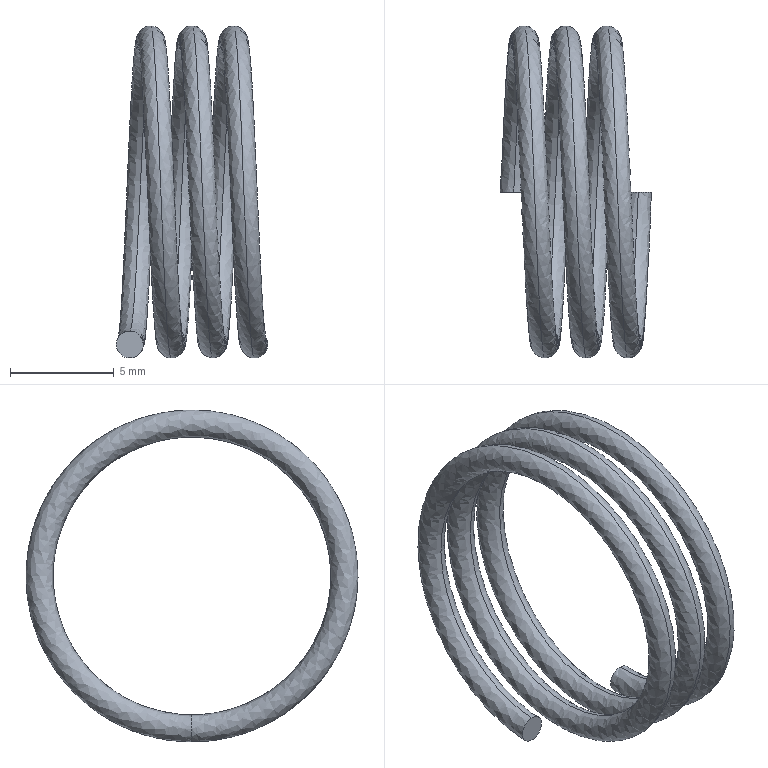Part | SolidWorks | features BaseBody 1, RefAxis 1 | 1 solid | 4 faces | box 7.3 x 16 x 16 mm | volume 183.83 mm3 | spline 2 | plane 2
STEP:
#1=CARTESIAN_POINT('',(-6.,0.,-8.));
#2=VERTEX_POINT('',#1);
#3=CARTESIAN_POINT('',(0.,0.,-8.));
#4=VERTEX_POINT('',#3);
#5=CARTESIAN_POINT('',(-6.,0.,-8.));
#6=CARTESIAN_POINT('',(-5.934,1.704,-8.));
#7=CARTESIAN_POINT('',(-5.866,3.324,-7.474));
#8=CARTESIAN_POINT('',(-5.8,4.702,-6.472));
#9=CARTESIAN_POINT('',(-5.734,6.081,-5.471));
#10=CARTESIAN_POINT('',(-5.666,7.082,-4.092));
#11=CARTESIAN_POINT('',(-5.6,7.608,-2.472));
#12=CARTESIAN_POINT('',(-5.534,8.135,-0.8518));
#13=CARTESIAN_POINT('',(-5.466,8.135,0.8518));
#14=CARTESIAN_POINT('',(-5.4,7.608,2.472));
#15=CARTESIAN_POINT('',(-5.334,7.082,4.092));
#16=CARTESIAN_POINT('',(-5.266,6.081,5.471));
#17=CARTESIAN_POINT('',(-5.2,4.702,6.472));
#18=CARTESIAN_POINT('',(-5.134,3.324,7.474));
#19=CARTESIAN_POINT('',(-5.066,1.704,8.));
#20=CARTESIAN_POINT('',(-5.,0.,8.));
#21=CARTESIAN_POINT('',(-4.934,-1.704,8.));
#22=CARTESIAN_POINT('',(-4.866,-3.324,7.474));
#23=CARTESIAN_POINT('',(-4.8,-4.702,6.472));
#24=CARTESIAN_POINT('',(-4.734,-6.081,5.471));
#25=CARTESIAN_POINT('',(-4.666,-7.082,4.092));
#26=CARTESIAN_POINT('',(-4.6,-7.608,2.472));
#27=CARTESIAN_POINT('',(-4.534,-8.135,0.8518));
#28=CARTESIAN_POINT('',(-4.466,-8.135,-0.8518));
#29=CARTESIAN_POINT('',(-4.4,-7.608,-2.472));
#30=CARTESIAN_POINT('',(-4.334,-7.082,-4.092));
#31=CARTESIAN_POINT('',(-4.266,-6.081,-5.471));
#32=CARTESIAN_POINT('',(-4.2,-4.702,-6.472));
#33=CARTESIAN_POINT('',(-4.134,-3.324,-7.474));
#34=CARTESIAN_POINT('',(-4.066,-1.704,-8.));
#35=CARTESIAN_POINT('',(-4.,0.,-8.));
#36=CARTESIAN_POINT('',(-3.934,1.704,-8.));
#37=CARTESIAN_POINT('',(-3.866,3.324,-7.474));
#38=CARTESIAN_POINT('',(-3.8,4.702,-6.472));
#39=CARTESIAN_POINT('',(-3.734,6.081,-5.471));
#40=CARTESIAN_POINT('',(-3.666,7.082,-4.092));
#41=CARTESIAN_POINT('',(-3.6,7.608,-2.472));
#42=CARTESIAN_POINT('',(-3.534,8.135,-0.8518));
#43=CARTESIAN_POINT('',(-3.466,8.135,0.8518));
#44=CARTESIAN_POINT('',(-3.4,7.608,2.472));
#45=CARTESIAN_POINT('',(-3.334,7.082,4.092));
#46=CARTESIAN_POINT('',(-3.266,6.081,5.471));
#47=CARTESIAN_POINT('',(-3.2,4.702,6.472));
#48=CARTESIAN_POINT('',(-3.134,3.324,7.474));
#49=CARTESIAN_POINT('',(-3.066,1.704,8.));
#50=CARTESIAN_POINT('',(-3.,0.,8.));
#51=CARTESIAN_POINT('',(-2.934,-1.704,8.));
#52=CARTESIAN_POINT('',(-2.866,-3.324,7.474));
#53=CARTESIAN_POINT('',(-2.8,-4.702,6.472));
#54=CARTESIAN_POINT('',(-2.734,-6.081,5.471));
#55=CARTESIAN_POINT('',(-2.666,-7.082,4.092));
#56=CARTESIAN_POINT('',(-2.6,-7.608,2.472));
#57=CARTESIAN_POINT('',(-2.534,-8.135,0.8518));
#58=CARTESIAN_POINT('',(-2.466,-8.135,-0.8518));
#59=CARTESIAN_POINT('',(-2.4,-7.608,-2.472));
#60=CARTESIAN_POINT('',(-2.334,-7.082,-4.092));
#61=CARTESIAN_POINT('',(-2.266,-6.081,-5.471));
#62=CARTESIAN_POINT('',(-2.2,-4.702,-6.472));
#63=CARTESIAN_POINT('',(-2.134,-3.324,-7.474));
#64=CARTESIAN_POINT('',(-2.066,-1.704,-8.));
#65=CARTESIAN_POINT('',(-2.,0.,-8.));
#66=CARTESIAN_POINT('',(-1.934,1.704,-8.));
#67=CARTESIAN_POINT('',(-1.866,3.324,-7.474));
#68=CARTESIAN_POINT('',(-1.8,4.702,-6.472));
#69=CARTESIAN_POINT('',(-1.734,6.081,-5.471));
#70=CARTESIAN_POINT('',(-1.666,7.082,-4.092));
#71=CARTESIAN_POINT('',(-1.6,7.608,-2.472));
#72=CARTESIAN_POINT('',(-1.534,8.135,-0.8518));
#73=CARTESIAN_POINT('',(-1.466,8.135,0.8518));
#74=CARTESIAN_POINT('',(-1.4,7.608,2.472));
#75=CARTESIAN_POINT('',(-1.334,7.082,4.092));
#76=CARTESIAN_POINT('',(-1.266,6.081,5.471));
#77=CARTESIAN_POINT('',(-1.2,4.702,6.472));
#78=CARTESIAN_POINT('',(-1.134,3.324,7.474));
#79=CARTESIAN_POINT('',(-1.066,1.704,8.));
#80=CARTESIAN_POINT('',(-1.,0.,8.));
#81=CARTESIAN_POINT('',(-0.9345,-1.704,8.));
#82=CARTESIAN_POINT('',(-0.8655,-3.324,7.474));
#83=CARTESIAN_POINT('',(-0.8,-4.702,6.472));
#84=CARTESIAN_POINT('',(-0.7345,-6.081,5.471));
#85=CARTESIAN_POINT('',(-0.6655,-7.082,4.092));
#86=CARTESIAN_POINT('',(-0.6,-7.608,2.472));
#87=CARTESIAN_POINT('',(-0.5345,-8.135,0.8518));
#88=CARTESIAN_POINT('',(-0.4655,-8.135,-0.8518));
#89=CARTESIAN_POINT('',(-0.4,-7.608,-2.472));
#90=CARTESIAN_POINT('',(-0.3345,-7.082,-4.092));
#91=CARTESIAN_POINT('',(-0.2655,-6.081,-5.471));
#92=CARTESIAN_POINT('',(-0.2,-4.702,-6.472));
#93=CARTESIAN_POINT('',(-0.1345,-3.324,-7.474));
#94=CARTESIAN_POINT('',(-0.06554,-1.704,-8.));
#95=CARTESIAN_POINT('',(0.,0.,-8.));
#96=(BOUNDED_CURVE()B_SPLINE_CURVE(3,(#5,#6,#7,#8,#9,#10,#11,#12,#13,#14,#15,#16,#17,#18,#19,#20,#21,#22,#23,#24,#25,#26,#27,#28,#29,#30,#31,#32,#33,#34,#35,#36,#37,#38,#39,#40,#41,#42,#43,#44,#45,#46,#47,#48,#49,#50,#51,#52,#53,#54,#55,#56,#57,#58,#59,#60,#61,#62,#63,#64,#65,#66,#67,#68,#69,#70,#71,#72,#73,#74,#75,#76,#77,#78,#79,#80,#81,#82,#83,#84,#85,#86,#87,#88,#89,#90,#91,#92,#93,#94,#95),.UNSPECIFIED.,.F.,.T.)B_SPLINE_CURVE_WITH_KNOTS((4,3,3,3,3,3,3,3,3,3,3,3,3,3,3,3,3,3,3,3,3,3,3,3,3,3,3,3,3,3,4),(0.,0.03333,0.06667,0.1,0.1333,0.1667,0.2,0.2333,0.2667,0.3,0.3333,0.3667,0.4,0.4333,0.4667,0.5,0.5333,0.5667,0.6,0.6333,0.6667,0.7,0.7333,0.7667,0.8,0.8333,0.8667,0.9,0.9333,0.9667,1.),.UNSPECIFIED.)CURVE()GEOMETRIC_REPRESENTATION_ITEM()RATIONAL_B_SPLINE_CURVE((1.,0.9674,0.9674,1.,0.9674,0.9674,1.,0.9674,0.9674,1.,0.9674,0.9674,1.,0.9674,0.9674,1.,0.9674,0.9674,1.,0.9674,0.9674,1.,0.9674,0.9674,1.,0.9674,0.9674,1.,0.9674,0.9674,1.,0.9674,0.9674,1.,0.9674,0.9674,1.,0.9674,0.9674,1.,0.9674,0.9674,1.,0.9674,0.9674,1.,0.9674,0.9674,1.,0.9674,0.9674,1.,0.9674,0.9674,1.,0.9674,0.9674,1.,0.9674,0.9674,1.,0.9674,0.9674,1.,0.9674,0.9674,1.,0.9674,0.9674,1.,0.9674,0.9674,1.,0.9674,0.9674,1.,0.9674,0.9674,1.,0.9674,0.9674,1.,0.9674,0.9674,1.,0.9674,0.9674,1.,0.9674,0.9674,1.))REPRESENTATION_ITEM(''));
#97=EDGE_CURVE('',#2,#4,#96,.T.);
#98=ORIENTED_EDGE('',*,*,#97,.F.);
#99=CARTESIAN_POINT('',(-6.,0.,-6.7));
#100=VERTEX_POINT('',#99);
#101=CARTESIAN_POINT('',(-6.,0.,-6.7));
#102=CARTESIAN_POINT('',(-7.3,0.,-6.7));
#103=CARTESIAN_POINT('',(-7.3,0.,-8.));
#104=CARTESIAN_POINT('',(-6.,0.,-8.));
#105=(BOUNDED_CURVE()B_SPLINE_CURVE(3,(#101,#102,#103,#104),.UNSPECIFIED.,.F.,.T.)B_SPLINE_CURVE_WITH_KNOTS((4,4),(0.,0.002032),.UNSPECIFIED.)CURVE()GEOMETRIC_REPRESENTATION_ITEM()RATIONAL_B_SPLINE_CURVE((1.,0.3333,0.3333,1.))REPRESENTATION_ITEM(''));
#106=EDGE_CURVE('',#100,#2,#105,.T.);
#107=ORIENTED_EDGE('',*,*,#106,.F.);
#108=CARTESIAN_POINT('',(0.,0.,-6.7));
#109=VERTEX_POINT('',#108);
#110=CARTESIAN_POINT('',(0.,0.,-6.7));
#111=CARTESIAN_POINT('',(-0.06554,-1.427,-6.7));
#112=CARTESIAN_POINT('',(-0.1345,-2.784,-6.259));
#113=CARTESIAN_POINT('',(-0.2,-3.938,-5.42));
#114=CARTESIAN_POINT('',(-0.2655,-5.092,-4.582));
#115=CARTESIAN_POINT('',(-0.3345,-5.931,-3.427));
#116=CARTESIAN_POINT('',(-0.4,-6.372,-2.07));
#117=CARTESIAN_POINT('',(-0.4655,-6.813,-0.7134));
#118=CARTESIAN_POINT('',(-0.5345,-6.813,0.7134));
#119=CARTESIAN_POINT('',(-0.6,-6.372,2.07));
#120=CARTESIAN_POINT('',(-0.6655,-5.931,3.427));
#121=CARTESIAN_POINT('',(-0.7345,-5.092,4.582));
#122=CARTESIAN_POINT('',(-0.8,-3.938,5.42));
#123=CARTESIAN_POINT('',(-0.8655,-2.784,6.259));
#124=CARTESIAN_POINT('',(-0.9345,-1.427,6.7));
#125=CARTESIAN_POINT('',(-1.,0.,6.7));
#126=CARTESIAN_POINT('',(-1.066,1.427,6.7));
#127=CARTESIAN_POINT('',(-1.134,2.784,6.259));
#128=CARTESIAN_POINT('',(-1.2,3.938,5.42));
#129=CARTESIAN_POINT('',(-1.266,5.092,4.582));
#130=CARTESIAN_POINT('',(-1.334,5.931,3.427));
#131=CARTESIAN_POINT('',(-1.4,6.372,2.07));
#132=CARTESIAN_POINT('',(-1.466,6.813,0.7134));
#133=CARTESIAN_POINT('',(-1.534,6.813,-0.7134));
#134=CARTESIAN_POINT('',(-1.6,6.372,-2.07));
#135=CARTESIAN_POINT('',(-1.666,5.931,-3.427));
#136=CARTESIAN_POINT('',(-1.734,5.092,-4.582));
#137=CARTESIAN_POINT('',(-1.8,3.938,-5.42));
#138=CARTESIAN_POINT('',(-1.866,2.784,-6.259));
#139=CARTESIAN_POINT('',(-1.934,1.427,-6.7));
#140=CARTESIAN_POINT('',(-2.,0.,-6.7));
#141=CARTESIAN_POINT('',(-2.066,-1.427,-6.7));
#142=CARTESIAN_POINT('',(-2.134,-2.784,-6.259));
#143=CARTESIAN_POINT('',(-2.2,-3.938,-5.42));
#144=CARTESIAN_POINT('',(-2.266,-5.092,-4.582));
#145=CARTESIAN_POINT('',(-2.334,-5.931,-3.427));
#146=CARTESIAN_POINT('',(-2.4,-6.372,-2.07));
#147=CARTESIAN_POINT('',(-2.466,-6.813,-0.7134));
#148=CARTESIAN_POINT('',(-2.534,-6.813,0.7134));
#149=CARTESIAN_POINT('',(-2.6,-6.372,2.07));
#150=CARTESIAN_POINT('',(-2.666,-5.931,3.427));
#151=CARTESIAN_POINT('',(-2.734,-5.092,4.582));
#152=CARTESIAN_POINT('',(-2.8,-3.938,5.42));
#153=CARTESIAN_POINT('',(-2.866,-2.784,6.259));
#154=CARTESIAN_POINT('',(-2.934,-1.427,6.7));
#155=CARTESIAN_POINT('',(-3.,0.,6.7));
#156=CARTESIAN_POINT('',(-3.066,1.427,6.7));
#157=CARTESIAN_POINT('',(-3.134,2.784,6.259));
#158=CARTESIAN_POINT('',(-3.2,3.938,5.42));
#159=CARTESIAN_POINT('',(-3.266,5.092,4.582));
#160=CARTESIAN_POINT('',(-3.334,5.931,3.427));
#161=CARTESIAN_POINT('',(-3.4,6.372,2.07));
#162=CARTESIAN_POINT('',(-3.466,6.813,0.7134));
#163=CARTESIAN_POINT('',(-3.534,6.813,-0.7134));
#164=CARTESIAN_POINT('',(-3.6,6.372,-2.07));
#165=CARTESIAN_POINT('',(-3.666,5.931,-3.427));
#166=CARTESIAN_POINT('',(-3.734,5.092,-4.582));
#167=CARTESIAN_POINT('',(-3.8,3.938,-5.42));
#168=CARTESIAN_POINT('',(-3.866,2.784,-6.259));
#169=CARTESIAN_POINT('',(-3.934,1.427,-6.7));
#170=CARTESIAN_POINT('',(-4.,0.,-6.7));
#171=CARTESIAN_POINT('',(-4.066,-1.427,-6.7));
#172=CARTESIAN_POINT('',(-4.134,-2.784,-6.259));
#173=CARTESIAN_POINT('',(-4.2,-3.938,-5.42));
#174=CARTESIAN_POINT('',(-4.266,-5.092,-4.582));
#175=CARTESIAN_POINT('',(-4.334,-5.931,-3.427));
#176=CARTESIAN_POINT('',(-4.4,-6.372,-2.07));
#177=CARTESIAN_POINT('',(-4.466,-6.813,-0.7134));
#178=CARTESIAN_POINT('',(-4.534,-6.813,0.7134));
#179=CARTESIAN_POINT('',(-4.6,-6.372,2.07));
#180=CARTESIAN_POINT('',(-4.666,-5.931,3.427));
#181=CARTESIAN_POINT('',(-4.734,-5.092,4.582));
#182=CARTESIAN_POINT('',(-4.8,-3.938,5.42));
#183=CARTESIAN_POINT('',(-4.866,-2.784,6.259));
#184=CARTESIAN_POINT('',(-4.934,-1.427,6.7));
#185=CARTESIAN_POINT('',(-5.,0.,6.7));
#186=CARTESIAN_POINT('',(-5.066,1.427,6.7));
#187=CARTESIAN_POINT('',(-5.134,2.784,6.259));
#188=CARTESIAN_POINT('',(-5.2,3.938,5.42));
#189=CARTESIAN_POINT('',(-5.266,5.092,4.582));
#190=CARTESIAN_POINT('',(-5.334,5.931,3.427));
#191=CARTESIAN_POINT('',(-5.4,6.372,2.07));
#192=CARTESIAN_POINT('',(-5.466,6.813,0.7134));
#193=CARTESIAN_POINT('',(-5.534,6.813,-0.7134));
#194=CARTESIAN_POINT('',(-5.6,6.372,-2.07));
#195=CARTESIAN_POINT('',(-5.666,5.931,-3.427));
#196=CARTESIAN_POINT('',(-5.734,5.092,-4.582));
#197=CARTESIAN_POINT('',(-5.8,3.938,-5.42));
#198=CARTESIAN_POINT('',(-5.866,2.784,-6.259));
#199=CARTESIAN_POINT('',(-5.934,1.427,-6.7));
#200=CARTESIAN_POINT('',(-6.,0.,-6.7));
#201=(BOUNDED_CURVE()B_SPLINE_CURVE(3,(#110,#111,#112,#113,#114,#115,#116,#117,#118,#119,#120,#121,#122,#123,#124,#125,#126,#127,#128,#129,#130,#131,#132,#133,#134,#135,#136,#137,#138,#139,#140,#141,#142,#143,#144,#145,#146,#147,#148,#149,#150,#151,#152,#153,#154,#155,#156,#157,#158,#159,#160,#161,#162,#163,#164,#165,#166,#167,#168,#169,#170,#171,#172,#173,#174,#175,#176,#177,#178,#179,#180,#181,#182,#183,#184,#185,#186,#187,#188,#189,#190,#191,#192,#193,#194,#195,#196,#197,#198,#199,#200),.UNSPECIFIED.,.F.,.F.)B_SPLINE_CURVE_WITH_KNOTS((4,3,3,3,3,3,3,3,3,3,3,3,3,3,3,3,3,3,3,3,3,3,3,3,3,3,3,3,3,3,4),(0.,0.03333,0.06667,0.1,0.1333,0.1667,0.2,0.2333,0.2667,0.3,0.3333,0.3667,0.4,0.4333,0.4667,0.5,0.5333,0.5667,0.6,0.6333,0.6667,0.7,0.7333,0.7667,0.8,0.8333,0.8667,0.9,0.9333,0.9667,1.),.UNSPECIFIED.)CURVE()GEOMETRIC_REPRESENTATION_ITEM()RATIONAL_B_SPLINE_CURVE((1.,0.9674,0.9674,1.,0.9674,0.9674,1.,0.9674,0.9674,1.,0.9674,0.9674,1.,0.9674,0.9674,1.,0.9674,0.9674,1.,0.9674,0.9674,1.,0.9674,0.9674,1.,0.9674,0.9674,1.,0.9674,0.9674,1.,0.9674,0.9674,1.,0.9674,0.9674,1.,0.9674,0.9674,1.,0.9674,0.9674,1.,0.9674,0.9674,1.,0.9674,0.9674,1.,0.9674,0.9674,1.,0.9674,0.9674,1.,0.9674,0.9674,1.,0.9674,0.9674,1.,0.9674,0.9674,1.,0.9674,0.9674,1.,0.9674,0.9674,1.,0.9674,0.9674,1.,0.9674,0.9674,1.,0.9674,0.9674,1.,0.9674,0.9674,1.,0.9674,0.9674,1.,0.9674,0.9674,1.,0.9674,0.9674,1.))REPRESENTATION_ITEM(''));
#202=EDGE_CURVE('',#109,#100,#201,.T.);
#203=ORIENTED_EDGE('',*,*,#202,.F.);
#204=CARTESIAN_POINT('',(0.,0.,-8.));
#205=CARTESIAN_POINT('',(-1.3,0.000000001,-8.));
#206=CARTESIAN_POINT('',(-1.3,0.,-6.7));
#207=CARTESIAN_POINT('',(0.,0.,-6.7));
#208=(BOUNDED_CURVE()B_SPLINE_CURVE(3,(#204,#205,#206,#207),.UNSPECIFIED.,.F.,.F.)B_SPLINE_CURVE_WITH_KNOTS((4,4),(0.,0.002032),.UNSPECIFIED.)CURVE()GEOMETRIC_REPRESENTATION_ITEM()RATIONAL_B_SPLINE_CURVE((1.,0.3333,0.3333,1.))REPRESENTATION_ITEM(''));
#209=EDGE_CURVE('',#4,#109,#208,.T.);
#210=ORIENTED_EDGE('',*,*,#209,.F.);
#211=EDGE_LOOP('',(#98,#107,#203,#210));
#212=FACE_OUTER_BOUND('',#211,.T.);
#213=CARTESIAN_POINT('',(0.,0.,-8.));
#214=CARTESIAN_POINT('',(-0.06554,-1.704,-8.));
#215=CARTESIAN_POINT('',(-0.1345,-3.324,-7.474));
#216=CARTESIAN_POINT('',(-0.2,-4.702,-6.472));
#217=CARTESIAN_POINT('',(-0.2655,-6.081,-5.471));
#218=CARTESIAN_POINT('',(-0.3345,-7.082,-4.092));
#219=CARTESIAN_POINT('',(-0.4,-7.608,-2.472));
#220=CARTESIAN_POINT('',(-0.4655,-8.135,-0.8518));
#221=CARTESIAN_POINT('',(-0.5345,-8.135,0.8518));
#222=CARTESIAN_POINT('',(-0.6,-7.608,2.472));
#223=CARTESIAN_POINT('',(-0.6655,-7.082,4.092));
#224=CARTESIAN_POINT('',(-0.7345,-6.081,5.471));
#225=CARTESIAN_POINT('',(-0.8,-4.702,6.472));
#226=CARTESIAN_POINT('',(-0.8655,-3.324,7.474));
#227=CARTESIAN_POINT('',(-0.9345,-1.704,8.));
#228=CARTESIAN_POINT('',(-1.,0.,8.));
#229=CARTESIAN_POINT('',(-1.066,1.704,8.));
#230=CARTESIAN_POINT('',(-1.134,3.324,7.474));
#231=CARTESIAN_POINT('',(-1.2,4.702,6.472));
#232=CARTESIAN_POINT('',(-1.266,6.081,5.471));
#233=CARTESIAN_POINT('',(-1.334,7.082,4.092));
#234=CARTESIAN_POINT('',(-1.4,7.608,2.472));
#235=CARTESIAN_POINT('',(-1.466,8.135,0.8518));
#236=CARTESIAN_POINT('',(-1.534,8.135,-0.8518));
#237=CARTESIAN_POINT('',(-1.6,7.608,-2.472));
#238=CARTESIAN_POINT('',(-1.666,7.082,-4.092));
#239=CARTESIAN_POINT('',(-1.734,6.081,-5.471));
#240=CARTESIAN_POINT('',(-1.8,4.702,-6.472));
#241=CARTESIAN_POINT('',(-1.866,3.324,-7.474));
#242=CARTESIAN_POINT('',(-1.934,1.704,-8.));
#243=CARTESIAN_POINT('',(-2.,0.,-8.));
#244=CARTESIAN_POINT('',(-2.066,-1.704,-8.));
#245=CARTESIAN_POINT('',(-2.134,-3.324,-7.474));
#246=CARTESIAN_POINT('',(-2.2,-4.702,-6.472));
#247=CARTESIAN_POINT('',(-2.266,-6.081,-5.471));
#248=CARTESIAN_POINT('',(-2.334,-7.082,-4.092));
#249=CARTESIAN_POINT('',(-2.4,-7.608,-2.472));
#250=CARTESIAN_POINT('',(-2.466,-8.135,-0.8518));
#251=CARTESIAN_POINT('',(-2.534,-8.135,0.8518));
#252=CARTESIAN_POINT('',(-2.6,-7.608,2.472));
#253=CARTESIAN_POINT('',(-2.666,-7.082,4.092));
#254=CARTESIAN_POINT('',(-2.734,-6.081,5.471));
#255=CARTESIAN_POINT('',(-2.8,-4.702,6.472));
#256=CARTESIAN_POINT('',(-2.866,-3.324,7.474));
#257=CARTESIAN_POINT('',(-2.934,-1.704,8.));
#258=CARTESIAN_POINT('',(-3.,0.,8.));
#259=CARTESIAN_POINT('',(-3.066,1.704,8.));
#260=CARTESIAN_POINT('',(-3.134,3.324,7.474));
#261=CARTESIAN_POINT('',(-3.2,4.702,6.472));
#262=CARTESIAN_POINT('',(-3.266,6.081,5.471));
#263=CARTESIAN_POINT('',(-3.334,7.082,4.092));
#264=CARTESIAN_POINT('',(-3.4,7.608,2.472));
#265=CARTESIAN_POINT('',(-3.466,8.135,0.8518));
#266=CARTESIAN_POINT('',(-3.534,8.135,-0.8518));
#267=CARTESIAN_POINT('',(-3.6,7.608,-2.472));
#268=CARTESIAN_POINT('',(-3.666,7.082,-4.092));
#269=CARTESIAN_POINT('',(-3.734,6.081,-5.471));
#270=CARTESIAN_POINT('',(-3.8,4.702,-6.472));
#271=CARTESIAN_POINT('',(-3.866,3.324,-7.474));
#272=CARTESIAN_POINT('',(-3.934,1.704,-8.));
#273=CARTESIAN_POINT('',(-4.,0.,-8.));
#274=CARTESIAN_POINT('',(-4.066,-1.704,-8.));
#275=CARTESIAN_POINT('',(-4.134,-3.324,-7.474));
#276=CARTESIAN_POINT('',(-4.2,-4.702,-6.472));
#277=CARTESIAN_POINT('',(-4.266,-6.081,-5.471));
#278=CARTESIAN_POINT('',(-4.334,-7.082,-4.092));
#279=CARTESIAN_POINT('',(-4.4,-7.608,-2.472));
#280=CARTESIAN_POINT('',(-4.466,-8.135,-0.8518));
#281=CARTESIAN_POINT('',(-4.534,-8.135,0.8518));
#282=CARTESIAN_POINT('',(-4.6,-7.608,2.472));
#283=CARTESIAN_POINT('',(-4.666,-7.082,4.092));
#284=CARTESIAN_POINT('',(-4.734,-6.081,5.471));
#285=CARTESIAN_POINT('',(-4.8,-4.702,6.472));
#286=CARTESIAN_POINT('',(-4.866,-3.324,7.474));
#287=CARTESIAN_POINT('',(-4.934,-1.704,8.));
#288=CARTESIAN_POINT('',(-5.,0.,8.));
#289=CARTESIAN_POINT('',(-5.066,1.704,8.));
#290=CARTESIAN_POINT('',(-5.134,3.324,7.474));
#291=CARTESIAN_POINT('',(-5.2,4.702,6.472));
#292=CARTESIAN_POINT('',(-5.266,6.081,5.471));
#293=CARTESIAN_POINT('',(-5.334,7.082,4.092));
#294=CARTESIAN_POINT('',(-5.4,7.608,2.472));
#295=CARTESIAN_POINT('',(-5.466,8.135,0.8518));
#296=CARTESIAN_POINT('',(-5.534,8.135,-0.8518));
#297=CARTESIAN_POINT('',(-5.6,7.608,-2.472));
#298=CARTESIAN_POINT('',(-5.666,7.082,-4.092));
#299=CARTESIAN_POINT('',(-5.734,6.081,-5.471));
#300=CARTESIAN_POINT('',(-5.8,4.702,-6.472));
#301=CARTESIAN_POINT('',(-5.866,3.324,-7.474));
#302=CARTESIAN_POINT('',(-5.934,1.704,-8.));
#303=CARTESIAN_POINT('',(-6.,0.,-8.));
#304=CARTESIAN_POINT('',(-1.3,0.,-8.));
#305=CARTESIAN_POINT('',(-1.366,-1.704,-8.));
#306=CARTESIAN_POINT('',(-1.434,-3.324,-7.474));
#307=CARTESIAN_POINT('',(-1.5,-4.702,-6.472));
#308=CARTESIAN_POINT('',(-1.566,-6.081,-5.471));
#309=CARTESIAN_POINT('',(-1.634,-7.082,-4.092));
#310=CARTESIAN_POINT('',(-1.7,-7.608,-2.472));
#311=CARTESIAN_POINT('',(-1.766,-8.135,-0.8518));
#312=CARTESIAN_POINT('',(-1.834,-8.135,0.8518));
#313=CARTESIAN_POINT('',(-1.9,-7.608,2.472));
#314=CARTESIAN_POINT('',(-1.966,-7.082,4.092));
#315=CARTESIAN_POINT('',(-2.034,-6.081,5.471));
#316=CARTESIAN_POINT('',(-2.1,-4.702,6.472));
#317=CARTESIAN_POINT('',(-2.166,-3.324,7.474));
#318=CARTESIAN_POINT('',(-2.234,-1.704,8.));
#319=CARTESIAN_POINT('',(-2.3,0.,8.));
#320=CARTESIAN_POINT('',(-2.366,1.704,8.));
#321=CARTESIAN_POINT('',(-2.434,3.324,7.474));
#322=CARTESIAN_POINT('',(-2.5,4.702,6.472));
#323=CARTESIAN_POINT('',(-2.566,6.081,5.471));
#324=CARTESIAN_POINT('',(-2.634,7.082,4.092));
#325=CARTESIAN_POINT('',(-2.7,7.608,2.472));
#326=CARTESIAN_POINT('',(-2.766,8.135,0.8518));
#327=CARTESIAN_POINT('',(-2.834,8.135,-0.8518));
#328=CARTESIAN_POINT('',(-2.9,7.608,-2.472));
#329=CARTESIAN_POINT('',(-2.966,7.082,-4.092));
#330=CARTESIAN_POINT('',(-3.034,6.081,-5.471));
#331=CARTESIAN_POINT('',(-3.1,4.702,-6.472));
#332=CARTESIAN_POINT('',(-3.166,3.324,-7.474));
#333=CARTESIAN_POINT('',(-3.234,1.704,-8.));
#334=CARTESIAN_POINT('',(-3.3,0.,-8.));
#335=CARTESIAN_POINT('',(-3.366,-1.704,-8.));
#336=CARTESIAN_POINT('',(-3.434,-3.324,-7.474));
#337=CARTESIAN_POINT('',(-3.5,-4.702,-6.472));
#338=CARTESIAN_POINT('',(-3.566,-6.081,-5.471));
#339=CARTESIAN_POINT('',(-3.634,-7.082,-4.092));
#340=CARTESIAN_POINT('',(-3.7,-7.608,-2.472));
#341=CARTESIAN_POINT('',(-3.766,-8.135,-0.8518));
#342=CARTESIAN_POINT('',(-3.834,-8.135,0.8518));
#343=CARTESIAN_POINT('',(-3.9,-7.608,2.472));
#344=CARTESIAN_POINT('',(-3.966,-7.082,4.092));
#345=CARTESIAN_POINT('',(-4.034,-6.081,5.471));
#346=CARTESIAN_POINT('',(-4.1,-4.702,6.472));
#347=CARTESIAN_POINT('',(-4.166,-3.324,7.474));
#348=CARTESIAN_POINT('',(-4.234,-1.704,8.));
#349=CARTESIAN_POINT('',(-4.3,0.,8.));
#350=CARTESIAN_POINT('',(-4.366,1.704,8.));
#351=CARTESIAN_POINT('',(-4.434,3.324,7.474));
#352=CARTESIAN_POINT('',(-4.5,4.702,6.472));
#353=CARTESIAN_POINT('',(-4.566,6.081,5.471));
#354=CARTESIAN_POINT('',(-4.634,7.082,4.092));
#355=CARTESIAN_POINT('',(-4.7,7.608,2.472));
#356=CARTESIAN_POINT('',(-4.766,8.135,0.8518));
#357=CARTESIAN_POINT('',(-4.834,8.135,-0.8518));
#358=CARTESIAN_POINT('',(-4.9,7.608,-2.472));
#359=CARTESIAN_POINT('',(-4.966,7.082,-4.092));
#360=CARTESIAN_POINT('',(-5.034,6.081,-5.471));
#361=CARTESIAN_POINT('',(-5.1,4.702,-6.472));
#362=CARTESIAN_POINT('',(-5.166,3.324,-7.474));
#363=CARTESIAN_POINT('',(-5.234,1.704,-8.));
#364=CARTESIAN_POINT('',(-5.3,0.,-8.));
#365=CARTESIAN_POINT('',(-5.366,-1.704,-8.));
#366=CARTESIAN_POINT('',(-5.434,-3.324,-7.474));
#367=CARTESIAN_POINT('',(-5.5,-4.702,-6.472));
#368=CARTESIAN_POINT('',(-5.566,-6.081,-5.471));
#369=CARTESIAN_POINT('',(-5.634,-7.082,-4.092));
#370=CARTESIAN_POINT('',(-5.7,-7.608,-2.472));
#371=CARTESIAN_POINT('',(-5.766,-8.135,-0.8518));
#372=CARTESIAN_POINT('',(-5.834,-8.135,0.8518));
#373=CARTESIAN_POINT('',(-5.9,-7.608,2.472));
#374=CARTESIAN_POINT('',(-5.966,-7.082,4.092));
#375=CARTESIAN_POINT('',(-6.034,-6.081,5.471));
#376=CARTESIAN_POINT('',(-6.1,-4.702,6.472));
#377=CARTESIAN_POINT('',(-6.166,-3.324,7.474));
#378=CARTESIAN_POINT('',(-6.234,-1.704,8.));
#379=CARTESIAN_POINT('',(-6.3,0.,8.));
#380=CARTESIAN_POINT('',(-6.366,1.704,8.));
#381=CARTESIAN_POINT('',(-6.434,3.324,7.474));
#382=CARTESIAN_POINT('',(-6.5,4.702,6.472));
#383=CARTESIAN_POINT('',(-6.566,6.081,5.471));
#384=CARTESIAN_POINT('',(-6.634,7.082,4.092));
#385=CARTESIAN_POINT('',(-6.7,7.608,2.472));
#386=CARTESIAN_POINT('',(-6.766,8.135,0.8518));
#387=CARTESIAN_POINT('',(-6.834,8.135,-0.8518));
#388=CARTESIAN_POINT('',(-6.9,7.608,-2.472));
#389=CARTESIAN_POINT('',(-6.966,7.082,-4.092));
#390=CARTESIAN_POINT('',(-7.034,6.081,-5.471));
#391=CARTESIAN_POINT('',(-7.1,4.702,-6.472));
#392=CARTESIAN_POINT('',(-7.166,3.324,-7.474));
#393=CARTESIAN_POINT('',(-7.234,1.704,-8.));
#394=CARTESIAN_POINT('',(-7.3,0.,-8.));
#395=CARTESIAN_POINT('',(-1.3,0.,-6.7));
#396=CARTESIAN_POINT('',(-1.366,-1.427,-6.7));
#397=CARTESIAN_POINT('',(-1.434,-2.784,-6.259));
#398=CARTESIAN_POINT('',(-1.5,-3.938,-5.42));
#399=CARTESIAN_POINT('',(-1.566,-5.092,-4.582));
#400=CARTESIAN_POINT('',(-1.634,-5.931,-3.427));
#401=CARTESIAN_POINT('',(-1.7,-6.372,-2.07));
#402=CARTESIAN_POINT('',(-1.766,-6.813,-0.7134));
#403=CARTESIAN_POINT('',(-1.834,-6.813,0.7134));
#404=CARTESIAN_POINT('',(-1.9,-6.372,2.07));
#405=CARTESIAN_POINT('',(-1.966,-5.931,3.427));
#406=CARTESIAN_POINT('',(-2.034,-5.092,4.582));
#407=CARTESIAN_POINT('',(-2.1,-3.938,5.42));
#408=CARTESIAN_POINT('',(-2.166,-2.784,6.259));
#409=CARTESIAN_POINT('',(-2.234,-1.427,6.7));
#410=CARTESIAN_POINT('',(-2.3,0.,6.7));
#411=CARTESIAN_POINT('',(-2.366,1.427,6.7));
#412=CARTESIAN_POINT('',(-2.434,2.784,6.259));
#413=CARTESIAN_POINT('',(-2.5,3.938,5.42));
#414=CARTESIAN_POINT('',(-2.566,5.092,4.582));
#415=CARTESIAN_POINT('',(-2.634,5.931,3.427));
#416=CARTESIAN_POINT('',(-2.7,6.372,2.07));
#417=CARTESIAN_POINT('',(-2.766,6.813,0.7134));
#418=CARTESIAN_POINT('',(-2.834,6.813,-0.7134));
#419=CARTESIAN_POINT('',(-2.9,6.372,-2.07));
#420=CARTESIAN_POINT('',(-2.966,5.931,-3.427));
#421=CARTESIAN_POINT('',(-3.034,5.092,-4.582));
#422=CARTESIAN_POINT('',(-3.1,3.938,-5.42));
#423=CARTESIAN_POINT('',(-3.166,2.784,-6.259));
#424=CARTESIAN_POINT('',(-3.234,1.427,-6.7));
#425=CARTESIAN_POINT('',(-3.3,0.,-6.7));
#426=CARTESIAN_POINT('',(-3.366,-1.427,-6.7));
#427=CARTESIAN_POINT('',(-3.434,-2.784,-6.259));
#428=CARTESIAN_POINT('',(-3.5,-3.938,-5.42));
#429=CARTESIAN_POINT('',(-3.566,-5.092,-4.582));
#430=CARTESIAN_POINT('',(-3.634,-5.931,-3.427));
#431=CARTESIAN_POINT('',(-3.7,-6.372,-2.07));
#432=CARTESIAN_POINT('',(-3.766,-6.813,-0.7134));
#433=CARTESIAN_POINT('',(-3.834,-6.813,0.7134));
#434=CARTESIAN_POINT('',(-3.9,-6.372,2.07));
#435=CARTESIAN_POINT('',(-3.966,-5.931,3.427));
#436=CARTESIAN_POINT('',(-4.034,-5.092,4.582));
#437=CARTESIAN_POINT('',(-4.1,-3.938,5.42));
#438=CARTESIAN_POINT('',(-4.166,-2.784,6.259));
#439=CARTESIAN_POINT('',(-4.234,-1.427,6.7));
#440=CARTESIAN_POINT('',(-4.3,0.,6.7));
#441=CARTESIAN_POINT('',(-4.366,1.427,6.7));
#442=CARTESIAN_POINT('',(-4.434,2.784,6.259));
#443=CARTESIAN_POINT('',(-4.5,3.938,5.42));
#444=CARTESIAN_POINT('',(-4.566,5.092,4.582));
#445=CARTESIAN_POINT('',(-4.634,5.931,3.427));
#446=CARTESIAN_POINT('',(-4.7,6.372,2.07));
#447=CARTESIAN_POINT('',(-4.766,6.813,0.7134));
#448=CARTESIAN_POINT('',(-4.834,6.813,-0.7134));
#449=CARTESIAN_POINT('',(-4.9,6.372,-2.07));
#450=CARTESIAN_POINT('',(-4.966,5.931,-3.427));
#451=CARTESIAN_POINT('',(-5.034,5.092,-4.582));
#452=CARTESIAN_POINT('',(-5.1,3.938,-5.42));
#453=CARTESIAN_POINT('',(-5.166,2.784,-6.259));
#454=CARTESIAN_POINT('',(-5.234,1.427,-6.7));
#455=CARTESIAN_POINT('',(-5.3,0.,-6.7));
#456=CARTESIAN_POINT('',(-5.366,-1.427,-6.7));
#457=CARTESIAN_POINT('',(-5.434,-2.784,-6.259));
#458=CARTESIAN_POINT('',(-5.5,-3.938,-5.42));
#459=CARTESIAN_POINT('',(-5.566,-5.092,-4.582));
#460=CARTESIAN_POINT('',(-5.634,-5.931,-3.427));
#461=CARTESIAN_POINT('',(-5.7,-6.372,-2.07));
#462=CARTESIAN_POINT('',(-5.766,-6.813,-0.7134));
#463=CARTESIAN_POINT('',(-5.834,-6.813,0.7134));
#464=CARTESIAN_POINT('',(-5.9,-6.372,2.07));
#465=CARTESIAN_POINT('',(-5.966,-5.931,3.427));
#466=CARTESIAN_POINT('',(-6.034,-5.092,4.582));
#467=CARTESIAN_POINT('',(-6.1,-3.938,5.42));
#468=CARTESIAN_POINT('',(-6.166,-2.784,6.259));
#469=CARTESIAN_POINT('',(-6.234,-1.427,6.7));
#470=CARTESIAN_POINT('',(-6.3,0.,6.7));
#471=CARTESIAN_POINT('',(-6.366,1.427,6.7));
#472=CARTESIAN_POINT('',(-6.434,2.784,6.259));
#473=CARTESIAN_POINT('',(-6.5,3.938,5.42));
#474=CARTESIAN_POINT('',(-6.566,5.092,4.582));
#475=CARTESIAN_POINT('',(-6.634,5.931,3.427));
#476=CARTESIAN_POINT('',(-6.7,6.372,2.07));
#477=CARTESIAN_POINT('',(-6.766,6.813,0.7134));
#478=CARTESIAN_POINT('',(-6.834,6.813,-0.7134));
#479=CARTESIAN_POINT('',(-6.9,6.372,-2.07));
#480=CARTESIAN_POINT('',(-6.966,5.931,-3.427));
#481=CARTESIAN_POINT('',(-7.034,5.092,-4.582));
#482=CARTESIAN_POINT('',(-7.1,3.938,-5.42));
#483=CARTESIAN_POINT('',(-7.166,2.784,-6.259));
#484=CARTESIAN_POINT('',(-7.234,1.427,-6.7));
#485=CARTESIAN_POINT('',(-7.3,0.,-6.7));
#486=CARTESIAN_POINT('',(0.,0.,-6.7));
#487=CARTESIAN_POINT('',(-0.06554,-1.427,-6.7));
#488=CARTESIAN_POINT('',(-0.1345,-2.784,-6.259));
#489=CARTESIAN_POINT('',(-0.2,-3.938,-5.42));
#490=CARTESIAN_POINT('',(-0.2655,-5.092,-4.582));
#491=CARTESIAN_POINT('',(-0.3345,-5.931,-3.427));
#492=CARTESIAN_POINT('',(-0.4,-6.372,-2.07));
#493=CARTESIAN_POINT('',(-0.4655,-6.813,-0.7134));
#494=CARTESIAN_POINT('',(-0.5345,-6.813,0.7134));
#495=CARTESIAN_POINT('',(-0.6,-6.372,2.07));
#496=CARTESIAN_POINT('',(-0.6655,-5.931,3.427));
#497=CARTESIAN_POINT('',(-0.7345,-5.092,4.582));
#498=CARTESIAN_POINT('',(-0.8,-3.938,5.42));
#499=CARTESIAN_POINT('',(-0.8655,-2.784,6.259));
#500=CARTESIAN_POINT('',(-0.9345,-1.427,6.7));
#501=CARTESIAN_POINT('',(-1.,0.,6.7));
#502=CARTESIAN_POINT('',(-1.066,1.427,6.7));
#503=CARTESIAN_POINT('',(-1.134,2.784,6.259));
#504=CARTESIAN_POINT('',(-1.2,3.938,5.42));
#505=CARTESIAN_POINT('',(-1.266,5.092,4.582));
#506=CARTESIAN_POINT('',(-1.334,5.931,3.427));
#507=CARTESIAN_POINT('',(-1.4,6.372,2.07));
#508=CARTESIAN_POINT('',(-1.466,6.813,0.7134));
#509=CARTESIAN_POINT('',(-1.534,6.813,-0.7134));
#510=CARTESIAN_POINT('',(-1.6,6.372,-2.07));
#511=CARTESIAN_POINT('',(-1.666,5.931,-3.427));
#512=CARTESIAN_POINT('',(-1.734,5.092,-4.582));
#513=CARTESIAN_POINT('',(-1.8,3.938,-5.42));
#514=CARTESIAN_POINT('',(-1.866,2.784,-6.259));
#515=CARTESIAN_POINT('',(-1.934,1.427,-6.7));
#516=CARTESIAN_POINT('',(-2.,0.,-6.7));
#517=CARTESIAN_POINT('',(-2.066,-1.427,-6.7));
#518=CARTESIAN_POINT('',(-2.134,-2.784,-6.259));
#519=CARTESIAN_POINT('',(-2.2,-3.938,-5.42));
#520=CARTESIAN_POINT('',(-2.266,-5.092,-4.582));
#521=CARTESIAN_POINT('',(-2.334,-5.931,-3.427));
#522=CARTESIAN_POINT('',(-2.4,-6.372,-2.07));
#523=CARTESIAN_POINT('',(-2.466,-6.813,-0.7134));
#524=CARTESIAN_POINT('',(-2.534,-6.813,0.7134));
#525=CARTESIAN_POINT('',(-2.6,-6.372,2.07));
#526=CARTESIAN_POINT('',(-2.666,-5.931,3.427));
#527=CARTESIAN_POINT('',(-2.734,-5.092,4.582));
#528=CARTESIAN_POINT('',(-2.8,-3.938,5.42));
#529=CARTESIAN_POINT('',(-2.866,-2.784,6.259));
#530=CARTESIAN_POINT('',(-2.934,-1.427,6.7));
#531=CARTESIAN_POINT('',(-3.,0.,6.7));
#532=CARTESIAN_POINT('',(-3.066,1.427,6.7));
#533=CARTESIAN_POINT('',(-3.134,2.784,6.259));
#534=CARTESIAN_POINT('',(-3.2,3.938,5.42));
#535=CARTESIAN_POINT('',(-3.266,5.092,4.582));
#536=CARTESIAN_POINT('',(-3.334,5.931,3.427));
#537=CARTESIAN_POINT('',(-3.4,6.372,2.07));
#538=CARTESIAN_POINT('',(-3.466,6.813,0.7134));
#539=CARTESIAN_POINT('',(-3.534,6.813,-0.7134));
#540=CARTESIAN_POINT('',(-3.6,6.372,-2.07));
#541=CARTESIAN_POINT('',(-3.666,5.931,-3.427));
#542=CARTESIAN_POINT('',(-3.734,5.092,-4.582));
#543=CARTESIAN_POINT('',(-3.8,3.938,-5.42));
#544=CARTESIAN_POINT('',(-3.866,2.784,-6.259));
#545=CARTESIAN_POINT('',(-3.934,1.427,-6.7));
#546=CARTESIAN_POINT('',(-4.,0.,-6.7));
#547=CARTESIAN_POINT('',(-4.066,-1.427,-6.7));
#548=CARTESIAN_POINT('',(-4.134,-2.784,-6.259));
#549=CARTESIAN_POINT('',(-4.2,-3.938,-5.42));
#550=CARTESIAN_POINT('',(-4.266,-5.092,-4.582));
#551=CARTESIAN_POINT('',(-4.334,-5.931,-3.427));
#552=CARTESIAN_POINT('',(-4.4,-6.372,-2.07));
#553=CARTESIAN_POINT('',(-4.466,-6.813,-0.7134));
#554=CARTESIAN_POINT('',(-4.534,-6.813,0.7134));
#555=CARTESIAN_POINT('',(-4.6,-6.372,2.07));
#556=CARTESIAN_POINT('',(-4.666,-5.931,3.427));
#557=CARTESIAN_POINT('',(-4.734,-5.092,4.582));
#558=CARTESIAN_POINT('',(-4.8,-3.938,5.42));
#559=CARTESIAN_POINT('',(-4.866,-2.784,6.259));
#560=CARTESIAN_POINT('',(-4.934,-1.427,6.7));
#561=CARTESIAN_POINT('',(-5.,0.,6.7));
#562=CARTESIAN_POINT('',(-5.066,1.427,6.7));
#563=CARTESIAN_POINT('',(-5.134,2.784,6.259));
#564=CARTESIAN_POINT('',(-5.2,3.938,5.42));
#565=CARTESIAN_POINT('',(-5.266,5.092,4.582));
#566=CARTESIAN_POINT('',(-5.334,5.931,3.427));
#567=CARTESIAN_POINT('',(-5.4,6.372,2.07));
#568=CARTESIAN_POINT('',(-5.466,6.813,0.7134));
#569=CARTESIAN_POINT('',(-5.534,6.813,-0.7134));
#570=CARTESIAN_POINT('',(-5.6,6.372,-2.07));
#571=CARTESIAN_POINT('',(-5.666,5.931,-3.427));
#572=CARTESIAN_POINT('',(-5.734,5.092,-4.582));
#573=CARTESIAN_POINT('',(-5.8,3.938,-5.42));
#574=CARTESIAN_POINT('',(-5.866,2.784,-6.259));
#575=CARTESIAN_POINT('',(-5.934,1.427,-6.7));
#576=CARTESIAN_POINT('',(-6.,0.,-6.7));
#577=(BOUNDED_SURFACE()B_SPLINE_SURFACE(3,3,((#213,#214,#215,#216,#217,#218,#219,#220,#221,#222,#223,#224,#225,#226,#227,#228,#229,#230,#231,#232,#233,#234,#235,#236,#237,#238,#239,#240,#241,#242,#243,#244,#245,#246,#247,#248,#249,#250,#251,#252,#253,#254,#255,#256,#257,#258,#259,#260,#261,#262,#263,#264,#265,#266,#267,#268,#269,#270,#271,#272,#273,#274,#275,#276,#277,#278,#279,#280,#281,#282,#283,#284,#285,#286,#287,#288,#289,#290,#291,#292,#293,#294,#295,#296,#297,#298,#299,#300,#301,#302,#303),(#304,#305,#306,#307,#308,#309,#310,#311,#312,#313,#314,#315,#316,#317,#318,#319,#320,#321,#322,#323,#324,#325,#326,#327,#328,#329,#330,#331,#332,#333,#334,#335,#336,#337,#338,#339,#340,#341,#342,#343,#344,#345,#346,#347,#348,#349,#350,#351,#352,#353,#354,#355,#356,#357,#358,#359,#360,#361,#362,#363,#364,#365,#366,#367,#368,#369,#370,#371,#372,#373,#374,#375,#376,#377,#378,#379,#380,#381,#382,#383,#384,#385,#386,#387,#388,#389,#390,#391,#392,#393,#394),(#395,#396,#397,#398,#399,#400,#401,#402,#403,#404,#405,#406,#407,#408,#409,#410,#411,#412,#413,#414,#415,#416,#417,#418,#419,#420,#421,#422,#423,#424,#425,#426,#427,#428,#429,#430,#431,#432,#433,#434,#435,#436,#437,#438,#439,#440,#441,#442,#443,#444,#445,#446,#447,#448,#449,#450,#451,#452,#453,#454,#455,#456,#457,#458,#459,#460,#461,#462,#463,#464,#465,#466,#467,#468,#469,#470,#471,#472,#473,#474,#475,#476,#477,#478,#479,#480,#481,#482,#483,#484,#485),(#486,#487,#488,#489,#490,#491,#492,#493,#494,#495,#496,#497,#498,#499,#500,#501,#502,#503,#504,#505,#506,#507,#508,#509,#510,#511,#512,#513,#514,#515,#516,#517,#518,#519,#520,#521,#522,#523,#524,#525,#526,#527,#528,#529,#530,#531,#532,#533,#534,#535,#536,#537,#538,#539,#540,#541,#542,#543,#544,#545,#546,#547,#548,#549,#550,#551,#552,#553,#554,#555,#556,#557,#558,#559,#560,#561,#562,#563,#564,#565,#566,#567,#568,#569,#570,#571,#572,#573,#574,#575,#576)),.UNSPECIFIED.,.F.,.F.,.F.)B_SPLINE_SURFACE_WITH_KNOTS((4,4),(4,3,3,3,3,3,3,3,3,3,3,3,3,3,3,3,3,3,3,3,3,3,3,3,3,3,3,3,3,3,4),(0.5,1.),(0.,0.03333,0.06667,0.1,0.1333,0.1667,0.2,0.2333,0.2667,0.3,0.3333,0.3667,0.4,0.4333,0.4667,0.5,0.5333,0.5667,0.6,0.6333,0.6667,0.7,0.7333,0.7667,0.8,0.8333,0.8667,0.9,0.9333,0.9667,1.),.UNSPECIFIED.)GEOMETRIC_REPRESENTATION_ITEM()RATIONAL_B_SPLINE_SURFACE(((1.,0.9674,0.9674,1.,0.9674,0.9674,1.,0.9674,0.9674,1.,0.9674,0.9674,1.,0.9674,0.9674,1.,0.9674,0.9674,1.,0.9674,0.9674,1.,0.9674,0.9674,1.,0.9674,0.9674,1.,0.9674,0.9674,1.,0.9674,0.9674,1.,0.9674,0.9674,1.,0.9674,0.9674,1.,0.9674,0.9674,1.,0.9674,0.9674,1.,0.9674,0.9674,1.,0.9674,0.9674,1.,0.9674,0.9674,1.,0.9674,0.9674,1.,0.9674,0.9674,1.,0.9674,0.9674,1.,0.9674,0.9674,1.,0.9674,0.9674,1.,0.9674,0.9674,1.,0.9674,0.9674,1.,0.9674,0.9674,1.,0.9674,0.9674,1.,0.9674,0.9674,1.,0.9674,0.9674,1.,0.9674,0.9674,1.),(0.3333,0.3225,0.3225,0.3333,0.3225,0.3225,0.3333,0.3225,0.3225,0.3333,0.3225,0.3225,0.3333,0.3225,0.3225,0.3333,0.3225,0.3225,0.3333,0.3225,0.3225,0.3333,0.3225,0.3225,0.3333,0.3225,0.3225,0.3333,0.3225,0.3225,0.3333,0.3225,0.3225,0.3333,0.3225,0.3225,0.3333,0.3225,0.3225,0.3333,0.3225,0.3225,0.3333,0.3225,0.3225,0.3333,0.3225,0.3225,0.3333,0.3225,0.3225,0.3333,0.3225,0.3225,0.3333,0.3225,0.3225,0.3333,0.3225,0.3225,0.3333,0.3225,0.3225,0.3333,0.3225,0.3225,0.3333,0.3225,0.3225,0.3333,0.3225,0.3225,0.3333,0.3225,0.3225,0.3333,0.3225,0.3225,0.3333,0.3225,0.3225,0.3333,0.3225,0.3225,0.3333,0.3225,0.3225,0.3333,0.3225,0.3225,0.3333),(0.3333,0.3225,0.3225,0.3333,0.3225,0.3225,0.3333,0.3225,0.3225,0.3333,0.3225,0.3225,0.3333,0.3225,0.3225,0.3333,0.3225,0.3225,0.3333,0.3225,0.3225,0.3333,0.3225,0.3225,0.3333,0.3225,0.3225,0.3333,0.3225,0.3225,0.3333,0.3225,0.3225,0.3333,0.3225,0.3225,0.3333,0.3225,0.3225,0.3333,0.3225,0.3225,0.3333,0.3225,0.3225,0.3333,0.3225,0.3225,0.3333,0.3225,0.3225,0.3333,0.3225,0.3225,0.3333,0.3225,0.3225,0.3333,0.3225,0.3225,0.3333,0.3225,0.3225,0.3333,0.3225,0.3225,0.3333,0.3225,0.3225,0.3333,0.3225,0.3225,0.3333,0.3225,0.3225,0.3333,0.3225,0.3225,0.3333,0.3225,0.3225,0.3333,0.3225,0.3225,0.3333,0.3225,0.3225,0.3333,0.3225,0.3225,0.3333),(1.,0.9674,0.9674,1.,0.9674,0.9674,1.,0.9674,0.9674,1.,0.9674,0.9674,1.,0.9674,0.9674,1.,0.9674,0.9674,1.,0.9674,0.9674,1.,0.9674,0.9674,1.,0.9674,0.9674,1.,0.9674,0.9674,1.,0.9674,0.9674,1.,0.9674,0.9674,1.,0.9674,0.9674,1.,0.9674,0.9674,1.,0.9674,0.9674,1.,0.9674,0.9674,1.,0.9674,0.9674,1.,0.9674,0.9674,1.,0.9674,0.9674,1.,0.9674,0.9674,1.,0.9674,0.9674,1.,0.9674,0.9674,1.,0.9674,0.9674,1.,0.9674,0.9674,1.,0.9674,0.9674,1.,0.9674,0.9674,1.,0.9674,0.9674,1.,0.9674,0.9674,1.,0.9674,0.9674,1.,0.9674,0.9674,1.)))REPRESENTATION_ITEM('')SURFACE());
#578=ADVANCED_FACE('',(#212),#577,.F.);
#579=ORIENTED_EDGE('',*,*,#209,.T.);
#580=CARTESIAN_POINT('',(0.,0.,-8.));
#581=CARTESIAN_POINT('',(1.3,0.,-8.));
#582=CARTESIAN_POINT('',(1.3,0.,-6.7));
#583=CARTESIAN_POINT('',(0.,0.,-6.7));
#584=(BOUNDED_CURVE()B_SPLINE_CURVE(3,(#580,#581,#582,#583),.UNSPECIFIED.,.F.,.F.)B_SPLINE_CURVE_WITH_KNOTS((4,4),(0.,0.002032),.UNSPECIFIED.)CURVE()GEOMETRIC_REPRESENTATION_ITEM()RATIONAL_B_SPLINE_CURVE((1.,0.3333,0.3333,1.))REPRESENTATION_ITEM(''));
#585=EDGE_CURVE('',#4,#109,#584,.T.);
#586=ORIENTED_EDGE('',*,*,#585,.F.);
#587=EDGE_LOOP('',(#579,#586));
#588=FACE_OUTER_BOUND('',#587,.T.);
#589=CARTESIAN_POINT('',(0.,0.,-8.));
#590=DIRECTION('',(0.,-1.,0.));
#591=DIRECTION('',(0.,0.,-1.));
#592=AXIS2_PLACEMENT_3D('',#589,#590,#591);
#593=PLANE('',#592);
#594=ADVANCED_FACE('',(#588),#593,.F.);
#595=ORIENTED_EDGE('',*,*,#585,.T.);
#596=ORIENTED_EDGE('',*,*,#202,.T.);
#597=CARTESIAN_POINT('',(-6.,0.,-8.));
#598=CARTESIAN_POINT('',(-4.7,-0.000000001,-8.));
#599=CARTESIAN_POINT('',(-4.7,0.,-6.7));
#600=CARTESIAN_POINT('',(-6.,0.,-6.7));
#601=(BOUNDED_CURVE()B_SPLINE_CURVE(3,(#597,#598,#599,#600),.UNSPECIFIED.,.F.,.F.)B_SPLINE_CURVE_WITH_KNOTS((4,4),(0.,0.002032),.UNSPECIFIED.)CURVE()GEOMETRIC_REPRESENTATION_ITEM()RATIONAL_B_SPLINE_CURVE((1.,0.3333,0.3333,1.))REPRESENTATION_ITEM(''));
#602=EDGE_CURVE('',#2,#100,#601,.T.);
#603=ORIENTED_EDGE('',*,*,#602,.F.);
#604=ORIENTED_EDGE('',*,*,#97,.T.);
#605=EDGE_LOOP('',(#595,#596,#603,#604));
#606=FACE_OUTER_BOUND('',#605,.T.);
#607=CARTESIAN_POINT('',(0.,0.,-6.7));
#608=CARTESIAN_POINT('',(-0.06554,-1.427,-6.7));
#609=CARTESIAN_POINT('',(-0.1345,-2.784,-6.259));
#610=CARTESIAN_POINT('',(-0.2,-3.938,-5.42));
#611=CARTESIAN_POINT('',(-0.2655,-5.092,-4.582));
#612=CARTESIAN_POINT('',(-0.3345,-5.931,-3.427));
#613=CARTESIAN_POINT('',(-0.4,-6.372,-2.07));
#614=CARTESIAN_POINT('',(-0.4655,-6.813,-0.7134));
#615=CARTESIAN_POINT('',(-0.5345,-6.813,0.7134));
#616=CARTESIAN_POINT('',(-0.6,-6.372,2.07));
#617=CARTESIAN_POINT('',(-0.6655,-5.931,3.427));
#618=CARTESIAN_POINT('',(-0.7345,-5.092,4.582));
#619=CARTESIAN_POINT('',(-0.8,-3.938,5.42));
#620=CARTESIAN_POINT('',(-0.8655,-2.784,6.259));
#621=CARTESIAN_POINT('',(-0.9345,-1.427,6.7));
#622=CARTESIAN_POINT('',(-1.,0.,6.7));
#623=CARTESIAN_POINT('',(-1.066,1.427,6.7));
#624=CARTESIAN_POINT('',(-1.134,2.784,6.259));
#625=CARTESIAN_POINT('',(-1.2,3.938,5.42));
#626=CARTESIAN_POINT('',(-1.266,5.092,4.582));
#627=CARTESIAN_POINT('',(-1.334,5.931,3.427));
#628=CARTESIAN_POINT('',(-1.4,6.372,2.07));
#629=CARTESIAN_POINT('',(-1.466,6.813,0.7134));
#630=CARTESIAN_POINT('',(-1.534,6.813,-0.7134));
#631=CARTESIAN_POINT('',(-1.6,6.372,-2.07));
#632=CARTESIAN_POINT('',(-1.666,5.931,-3.427));
#633=CARTESIAN_POINT('',(-1.734,5.092,-4.582));
#634=CARTESIAN_POINT('',(-1.8,3.938,-5.42));
#635=CARTESIAN_POINT('',(-1.866,2.784,-6.259));
#636=CARTESIAN_POINT('',(-1.934,1.427,-6.7));
#637=CARTESIAN_POINT('',(-2.,0.,-6.7));
#638=CARTESIAN_POINT('',(-2.066,-1.427,-6.7));
#639=CARTESIAN_POINT('',(-2.134,-2.784,-6.259));
#640=CARTESIAN_POINT('',(-2.2,-3.938,-5.42));
#641=CARTESIAN_POINT('',(-2.266,-5.092,-4.582));
#642=CARTESIAN_POINT('',(-2.334,-5.931,-3.427));
#643=CARTESIAN_POINT('',(-2.4,-6.372,-2.07));
#644=CARTESIAN_POINT('',(-2.466,-6.813,-0.7134));
#645=CARTESIAN_POINT('',(-2.534,-6.813,0.7134));
#646=CARTESIAN_POINT('',(-2.6,-6.372,2.07));
#647=CARTESIAN_POINT('',(-2.666,-5.931,3.427));
#648=CARTESIAN_POINT('',(-2.734,-5.092,4.582));
#649=CARTESIAN_POINT('',(-2.8,-3.938,5.42));
#650=CARTESIAN_POINT('',(-2.866,-2.784,6.259));
#651=CARTESIAN_POINT('',(-2.934,-1.427,6.7));
#652=CARTESIAN_POINT('',(-3.,0.,6.7));
#653=CARTESIAN_POINT('',(-3.066,1.427,6.7));
#654=CARTESIAN_POINT('',(-3.134,2.784,6.259));
#655=CARTESIAN_POINT('',(-3.2,3.938,5.42));
#656=CARTESIAN_POINT('',(-3.266,5.092,4.582));
#657=CARTESIAN_POINT('',(-3.334,5.931,3.427));
#658=CARTESIAN_POINT('',(-3.4,6.372,2.07));
#659=CARTESIAN_POINT('',(-3.466,6.813,0.7134));
#660=CARTESIAN_POINT('',(-3.534,6.813,-0.7134));
#661=CARTESIAN_POINT('',(-3.6,6.372,-2.07));
#662=CARTESIAN_POINT('',(-3.666,5.931,-3.427));
#663=CARTESIAN_POINT('',(-3.734,5.092,-4.582));
#664=CARTESIAN_POINT('',(-3.8,3.938,-5.42));
#665=CARTESIAN_POINT('',(-3.866,2.784,-6.259));
#666=CARTESIAN_POINT('',(-3.934,1.427,-6.7));
#667=CARTESIAN_POINT('',(-4.,0.,-6.7));
#668=CARTESIAN_POINT('',(-4.066,-1.427,-6.7));
#669=CARTESIAN_POINT('',(-4.134,-2.784,-6.259));
#670=CARTESIAN_POINT('',(-4.2,-3.938,-5.42));
#671=CARTESIAN_POINT('',(-4.266,-5.092,-4.582));
#672=CARTESIAN_POINT('',(-4.334,-5.931,-3.427));
#673=CARTESIAN_POINT('',(-4.4,-6.372,-2.07));
#674=CARTESIAN_POINT('',(-4.466,-6.813,-0.7134));
#675=CARTESIAN_POINT('',(-4.534,-6.813,0.7134));
#676=CARTESIAN_POINT('',(-4.6,-6.372,2.07));
#677=CARTESIAN_POINT('',(-4.666,-5.931,3.427));
#678=CARTESIAN_POINT('',(-4.734,-5.092,4.582));
#679=CARTESIAN_POINT('',(-4.8,-3.938,5.42));
#680=CARTESIAN_POINT('',(-4.866,-2.784,6.259));
#681=CARTESIAN_POINT('',(-4.934,-1.427,6.7));
#682=CARTESIAN_POINT('',(-5.,0.,6.7));
#683=CARTESIAN_POINT('',(-5.066,1.427,6.7));
#684=CARTESIAN_POINT('',(-5.134,2.784,6.259));
#685=CARTESIAN_POINT('',(-5.2,3.938,5.42));
#686=CARTESIAN_POINT('',(-5.266,5.092,4.582));
#687=CARTESIAN_POINT('',(-5.334,5.931,3.427));
#688=CARTESIAN_POINT('',(-5.4,6.372,2.07));
#689=CARTESIAN_POINT('',(-5.466,6.813,0.7134));
#690=CARTESIAN_POINT('',(-5.534,6.813,-0.7134));
#691=CARTESIAN_POINT('',(-5.6,6.372,-2.07));
#692=CARTESIAN_POINT('',(-5.666,5.931,-3.427));
#693=CARTESIAN_POINT('',(-5.734,5.092,-4.582));
#694=CARTESIAN_POINT('',(-5.8,3.938,-5.42));
#695=CARTESIAN_POINT('',(-5.866,2.784,-6.259));
#696=CARTESIAN_POINT('',(-5.934,1.427,-6.7));
#697=CARTESIAN_POINT('',(-6.,0.,-6.7));
#698=CARTESIAN_POINT('',(1.3,0.,-6.7));
#699=CARTESIAN_POINT('',(1.234,-1.427,-6.7));
#700=CARTESIAN_POINT('',(1.166,-2.784,-6.259));
#701=CARTESIAN_POINT('',(1.1,-3.938,-5.42));
#702=CARTESIAN_POINT('',(1.034,-5.092,-4.582));
#703=CARTESIAN_POINT('',(0.9655,-5.931,-3.427));
#704=CARTESIAN_POINT('',(0.9,-6.372,-2.07));
#705=CARTESIAN_POINT('',(0.8345,-6.813,-0.7134));
#706=CARTESIAN_POINT('',(0.7655,-6.813,0.7134));
#707=CARTESIAN_POINT('',(0.7,-6.372,2.07));
#708=CARTESIAN_POINT('',(0.6345,-5.931,3.427));
#709=CARTESIAN_POINT('',(0.5655,-5.092,4.582));
#710=CARTESIAN_POINT('',(0.5,-3.938,5.42));
#711=CARTESIAN_POINT('',(0.4345,-2.784,6.259));
#712=CARTESIAN_POINT('',(0.3655,-1.427,6.7));
#713=CARTESIAN_POINT('',(0.3,0.,6.7));
#714=CARTESIAN_POINT('',(0.2345,1.427,6.7));
#715=CARTESIAN_POINT('',(0.1655,2.784,6.259));
#716=CARTESIAN_POINT('',(0.1,3.938,5.42));
#717=CARTESIAN_POINT('',(0.03446,5.092,4.582));
#718=CARTESIAN_POINT('',(-0.03446,5.931,3.427));
#719=CARTESIAN_POINT('',(-0.1,6.372,2.07));
#720=CARTESIAN_POINT('',(-0.1655,6.813,0.7134));
#721=CARTESIAN_POINT('',(-0.2345,6.813,-0.7134));
#722=CARTESIAN_POINT('',(-0.3,6.372,-2.07));
#723=CARTESIAN_POINT('',(-0.3655,5.931,-3.427));
#724=CARTESIAN_POINT('',(-0.4345,5.092,-4.582));
#725=CARTESIAN_POINT('',(-0.5,3.938,-5.42));
#726=CARTESIAN_POINT('',(-0.5655,2.784,-6.259));
#727=CARTESIAN_POINT('',(-0.6345,1.427,-6.7));
#728=CARTESIAN_POINT('',(-0.7,0.,-6.7));
#729=CARTESIAN_POINT('',(-0.7655,-1.427,-6.7));
#730=CARTESIAN_POINT('',(-0.8345,-2.784,-6.259));
#731=CARTESIAN_POINT('',(-0.9,-3.938,-5.42));
#732=CARTESIAN_POINT('',(-0.9655,-5.092,-4.582));
#733=CARTESIAN_POINT('',(-1.034,-5.931,-3.427));
#734=CARTESIAN_POINT('',(-1.1,-6.372,-2.07));
#735=CARTESIAN_POINT('',(-1.166,-6.813,-0.7134));
#736=CARTESIAN_POINT('',(-1.234,-6.813,0.7134));
#737=CARTESIAN_POINT('',(-1.3,-6.372,2.07));
#738=CARTESIAN_POINT('',(-1.366,-5.931,3.427));
#739=CARTESIAN_POINT('',(-1.434,-5.092,4.582));
#740=CARTESIAN_POINT('',(-1.5,-3.938,5.42));
#741=CARTESIAN_POINT('',(-1.566,-2.784,6.259));
#742=CARTESIAN_POINT('',(-1.634,-1.427,6.7));
#743=CARTESIAN_POINT('',(-1.7,0.,6.7));
#744=CARTESIAN_POINT('',(-1.766,1.427,6.7));
#745=CARTESIAN_POINT('',(-1.834,2.784,6.259));
#746=CARTESIAN_POINT('',(-1.9,3.938,5.42));
#747=CARTESIAN_POINT('',(-1.966,5.092,4.582));
#748=CARTESIAN_POINT('',(-2.034,5.931,3.427));
#749=CARTESIAN_POINT('',(-2.1,6.372,2.07));
#750=CARTESIAN_POINT('',(-2.166,6.813,0.7134));
#751=CARTESIAN_POINT('',(-2.234,6.813,-0.7134));
#752=CARTESIAN_POINT('',(-2.3,6.372,-2.07));
#753=CARTESIAN_POINT('',(-2.366,5.931,-3.427));
#754=CARTESIAN_POINT('',(-2.434,5.092,-4.582));
#755=CARTESIAN_POINT('',(-2.5,3.938,-5.42));
#756=CARTESIAN_POINT('',(-2.566,2.784,-6.259));
#757=CARTESIAN_POINT('',(-2.634,1.427,-6.7));
#758=CARTESIAN_POINT('',(-2.7,0.,-6.7));
#759=CARTESIAN_POINT('',(-2.766,-1.427,-6.7));
#760=CARTESIAN_POINT('',(-2.834,-2.784,-6.259));
#761=CARTESIAN_POINT('',(-2.9,-3.938,-5.42));
#762=CARTESIAN_POINT('',(-2.966,-5.092,-4.582));
#763=CARTESIAN_POINT('',(-3.034,-5.931,-3.427));
#764=CARTESIAN_POINT('',(-3.1,-6.372,-2.07));
#765=CARTESIAN_POINT('',(-3.166,-6.813,-0.7134));
#766=CARTESIAN_POINT('',(-3.234,-6.813,0.7134));
#767=CARTESIAN_POINT('',(-3.3,-6.372,2.07));
#768=CARTESIAN_POINT('',(-3.366,-5.931,3.427));
#769=CARTESIAN_POINT('',(-3.434,-5.092,4.582));
#770=CARTESIAN_POINT('',(-3.5,-3.938,5.42));
#771=CARTESIAN_POINT('',(-3.566,-2.784,6.259));
#772=CARTESIAN_POINT('',(-3.634,-1.427,6.7));
#773=CARTESIAN_POINT('',(-3.7,0.,6.7));
#774=CARTESIAN_POINT('',(-3.766,1.427,6.7));
#775=CARTESIAN_POINT('',(-3.834,2.784,6.259));
#776=CARTESIAN_POINT('',(-3.9,3.938,5.42));
#777=CARTESIAN_POINT('',(-3.966,5.092,4.582));
#778=CARTESIAN_POINT('',(-4.034,5.931,3.427));
#779=CARTESIAN_POINT('',(-4.1,6.372,2.07));
#780=CARTESIAN_POINT('',(-4.166,6.813,0.7134));
#781=CARTESIAN_POINT('',(-4.234,6.813,-0.7134));
#782=CARTESIAN_POINT('',(-4.3,6.372,-2.07));
#783=CARTESIAN_POINT('',(-4.366,5.931,-3.427));
#784=CARTESIAN_POINT('',(-4.434,5.092,-4.582));
#785=CARTESIAN_POINT('',(-4.5,3.938,-5.42));
#786=CARTESIAN_POINT('',(-4.566,2.784,-6.259));
#787=CARTESIAN_POINT('',(-4.634,1.427,-6.7));
#788=CARTESIAN_POINT('',(-4.7,0.,-6.7));
#789=CARTESIAN_POINT('',(1.3,0.,-8.));
#790=CARTESIAN_POINT('',(1.234,-1.704,-8.));
#791=CARTESIAN_POINT('',(1.166,-3.324,-7.474));
#792=CARTESIAN_POINT('',(1.1,-4.702,-6.472));
#793=CARTESIAN_POINT('',(1.034,-6.081,-5.471));
#794=CARTESIAN_POINT('',(0.9655,-7.082,-4.092));
#795=CARTESIAN_POINT('',(0.9,-7.608,-2.472));
#796=CARTESIAN_POINT('',(0.8345,-8.135,-0.8518));
#797=CARTESIAN_POINT('',(0.7655,-8.135,0.8518));
#798=CARTESIAN_POINT('',(0.7,-7.608,2.472));
#799=CARTESIAN_POINT('',(0.6345,-7.082,4.092));
#800=CARTESIAN_POINT('',(0.5655,-6.081,5.471));
#801=CARTESIAN_POINT('',(0.5,-4.702,6.472));
#802=CARTESIAN_POINT('',(0.4345,-3.324,7.474));
#803=CARTESIAN_POINT('',(0.3655,-1.704,8.));
#804=CARTESIAN_POINT('',(0.3,0.,8.));
#805=CARTESIAN_POINT('',(0.2345,1.704,8.));
#806=CARTESIAN_POINT('',(0.1655,3.324,7.474));
#807=CARTESIAN_POINT('',(0.1,4.702,6.472));
#808=CARTESIAN_POINT('',(0.03446,6.081,5.471));
#809=CARTESIAN_POINT('',(-0.03446,7.082,4.092));
#810=CARTESIAN_POINT('',(-0.1,7.608,2.472));
#811=CARTESIAN_POINT('',(-0.1655,8.135,0.8518));
#812=CARTESIAN_POINT('',(-0.2345,8.135,-0.8518));
#813=CARTESIAN_POINT('',(-0.3,7.608,-2.472));
#814=CARTESIAN_POINT('',(-0.3655,7.082,-4.092));
#815=CARTESIAN_POINT('',(-0.4345,6.081,-5.471));
#816=CARTESIAN_POINT('',(-0.5,4.702,-6.472));
#817=CARTESIAN_POINT('',(-0.5655,3.324,-7.474));
#818=CARTESIAN_POINT('',(-0.6345,1.704,-8.));
#819=CARTESIAN_POINT('',(-0.7,0.,-8.));
#820=CARTESIAN_POINT('',(-0.7655,-1.704,-8.));
#821=CARTESIAN_POINT('',(-0.8345,-3.324,-7.474));
#822=CARTESIAN_POINT('',(-0.9,-4.702,-6.472));
#823=CARTESIAN_POINT('',(-0.9655,-6.081,-5.471));
#824=CARTESIAN_POINT('',(-1.034,-7.082,-4.092));
#825=CARTESIAN_POINT('',(-1.1,-7.608,-2.472));
#826=CARTESIAN_POINT('',(-1.166,-8.135,-0.8518));
#827=CARTESIAN_POINT('',(-1.234,-8.135,0.8518));
#828=CARTESIAN_POINT('',(-1.3,-7.608,2.472));
#829=CARTESIAN_POINT('',(-1.366,-7.082,4.092));
#830=CARTESIAN_POINT('',(-1.434,-6.081,5.471));
#831=CARTESIAN_POINT('',(-1.5,-4.702,6.472));
#832=CARTESIAN_POINT('',(-1.566,-3.324,7.474));
#833=CARTESIAN_POINT('',(-1.634,-1.704,8.));
#834=CARTESIAN_POINT('',(-1.7,0.,8.));
#835=CARTESIAN_POINT('',(-1.766,1.704,8.));
#836=CARTESIAN_POINT('',(-1.834,3.324,7.474));
#837=CARTESIAN_POINT('',(-1.9,4.702,6.472));
#838=CARTESIAN_POINT('',(-1.966,6.081,5.471));
#839=CARTESIAN_POINT('',(-2.034,7.082,4.092));
#840=CARTESIAN_POINT('',(-2.1,7.608,2.472));
#841=CARTESIAN_POINT('',(-2.166,8.135,0.8518));
#842=CARTESIAN_POINT('',(-2.234,8.135,-0.8518));
#843=CARTESIAN_POINT('',(-2.3,7.608,-2.472));
#844=CARTESIAN_POINT('',(-2.366,7.082,-4.092));
#845=CARTESIAN_POINT('',(-2.434,6.081,-5.471));
#846=CARTESIAN_POINT('',(-2.5,4.702,-6.472));
#847=CARTESIAN_POINT('',(-2.566,3.324,-7.474));
#848=CARTESIAN_POINT('',(-2.634,1.704,-8.));
#849=CARTESIAN_POINT('',(-2.7,0.,-8.));
#850=CARTESIAN_POINT('',(-2.766,-1.704,-8.));
#851=CARTESIAN_POINT('',(-2.834,-3.324,-7.474));
#852=CARTESIAN_POINT('',(-2.9,-4.702,-6.472));
#853=CARTESIAN_POINT('',(-2.966,-6.081,-5.471));
#854=CARTESIAN_POINT('',(-3.034,-7.082,-4.092));
#855=CARTESIAN_POINT('',(-3.1,-7.608,-2.472));
#856=CARTESIAN_POINT('',(-3.166,-8.135,-0.8518));
#857=CARTESIAN_POINT('',(-3.234,-8.135,0.8518));
#858=CARTESIAN_POINT('',(-3.3,-7.608,2.472));
#859=CARTESIAN_POINT('',(-3.366,-7.082,4.092));
#860=CARTESIAN_POINT('',(-3.434,-6.081,5.471));
#861=CARTESIAN_POINT('',(-3.5,-4.702,6.472));
#862=CARTESIAN_POINT('',(-3.566,-3.324,7.474));
#863=CARTESIAN_POINT('',(-3.634,-1.704,8.));
#864=CARTESIAN_POINT('',(-3.7,0.,8.));
#865=CARTESIAN_POINT('',(-3.766,1.704,8.));
#866=CARTESIAN_POINT('',(-3.834,3.324,7.474));
#867=CARTESIAN_POINT('',(-3.9,4.702,6.472));
#868=CARTESIAN_POINT('',(-3.966,6.081,5.471));
#869=CARTESIAN_POINT('',(-4.034,7.082,4.092));
#870=CARTESIAN_POINT('',(-4.1,7.608,2.472));
#871=CARTESIAN_POINT('',(-4.166,8.135,0.8518));
#872=CARTESIAN_POINT('',(-4.234,8.135,-0.8518));
#873=CARTESIAN_POINT('',(-4.3,7.608,-2.472));
#874=CARTESIAN_POINT('',(-4.366,7.082,-4.092));
#875=CARTESIAN_POINT('',(-4.434,6.081,-5.471));
#876=CARTESIAN_POINT('',(-4.5,4.702,-6.472));
#877=CARTESIAN_POINT('',(-4.566,3.324,-7.474));
#878=CARTESIAN_POINT('',(-4.634,1.704,-8.));
#879=CARTESIAN_POINT('',(-4.7,0.,-8.));
#880=CARTESIAN_POINT('',(0.,0.,-8.));
#881=CARTESIAN_POINT('',(-0.06554,-1.704,-8.));
#882=CARTESIAN_POINT('',(-0.1345,-3.324,-7.474));
#883=CARTESIAN_POINT('',(-0.2,-4.702,-6.472));
#884=CARTESIAN_POINT('',(-0.2655,-6.081,-5.471));
#885=CARTESIAN_POINT('',(-0.3345,-7.082,-4.092));
#886=CARTESIAN_POINT('',(-0.4,-7.608,-2.472));
#887=CARTESIAN_POINT('',(-0.4655,-8.135,-0.8518));
#888=CARTESIAN_POINT('',(-0.5345,-8.135,0.8518));
#889=CARTESIAN_POINT('',(-0.6,-7.608,2.472));
#890=CARTESIAN_POINT('',(-0.6655,-7.082,4.092));
#891=CARTESIAN_POINT('',(-0.7345,-6.081,5.471));
#892=CARTESIAN_POINT('',(-0.8,-4.702,6.472));
#893=CARTESIAN_POINT('',(-0.8655,-3.324,7.474));
#894=CARTESIAN_POINT('',(-0.9345,-1.704,8.));
#895=CARTESIAN_POINT('',(-1.,0.,8.));
#896=CARTESIAN_POINT('',(-1.066,1.704,8.));
#897=CARTESIAN_POINT('',(-1.134,3.324,7.474));
#898=CARTESIAN_POINT('',(-1.2,4.702,6.472));
#899=CARTESIAN_POINT('',(-1.266,6.081,5.471));
#900=CARTESIAN_POINT('',(-1.334,7.082,4.092));
#901=CARTESIAN_POINT('',(-1.4,7.608,2.472));
#902=CARTESIAN_POINT('',(-1.466,8.135,0.8518));
#903=CARTESIAN_POINT('',(-1.534,8.135,-0.8518));
#904=CARTESIAN_POINT('',(-1.6,7.608,-2.472));
#905=CARTESIAN_POINT('',(-1.666,7.082,-4.092));
#906=CARTESIAN_POINT('',(-1.734,6.081,-5.471));
#907=CARTESIAN_POINT('',(-1.8,4.702,-6.472));
#908=CARTESIAN_POINT('',(-1.866,3.324,-7.474));
#909=CARTESIAN_POINT('',(-1.934,1.704,-8.));
#910=CARTESIAN_POINT('',(-2.,0.,-8.));
#911=CARTESIAN_POINT('',(-2.066,-1.704,-8.));
#912=CARTESIAN_POINT('',(-2.134,-3.324,-7.474));
#913=CARTESIAN_POINT('',(-2.2,-4.702,-6.472));
#914=CARTESIAN_POINT('',(-2.266,-6.081,-5.471));
#915=CARTESIAN_POINT('',(-2.334,-7.082,-4.092));
#916=CARTESIAN_POINT('',(-2.4,-7.608,-2.472));
#917=CARTESIAN_POINT('',(-2.466,-8.135,-0.8518));
#918=CARTESIAN_POINT('',(-2.534,-8.135,0.8518));
#919=CARTESIAN_POINT('',(-2.6,-7.608,2.472));
#920=CARTESIAN_POINT('',(-2.666,-7.082,4.092));
#921=CARTESIAN_POINT('',(-2.734,-6.081,5.471));
#922=CARTESIAN_POINT('',(-2.8,-4.702,6.472));
#923=CARTESIAN_POINT('',(-2.866,-3.324,7.474));
#924=CARTESIAN_POINT('',(-2.934,-1.704,8.));
#925=CARTESIAN_POINT('',(-3.,0.,8.));
#926=CARTESIAN_POINT('',(-3.066,1.704,8.));
#927=CARTESIAN_POINT('',(-3.134,3.324,7.474));
#928=CARTESIAN_POINT('',(-3.2,4.702,6.472));
#929=CARTESIAN_POINT('',(-3.266,6.081,5.471));
#930=CARTESIAN_POINT('',(-3.334,7.082,4.092));
#931=CARTESIAN_POINT('',(-3.4,7.608,2.472));
#932=CARTESIAN_POINT('',(-3.466,8.135,0.8518));
#933=CARTESIAN_POINT('',(-3.534,8.135,-0.8518));
#934=CARTESIAN_POINT('',(-3.6,7.608,-2.472));
#935=CARTESIAN_POINT('',(-3.666,7.082,-4.092));
#936=CARTESIAN_POINT('',(-3.734,6.081,-5.471));
#937=CARTESIAN_POINT('',(-3.8,4.702,-6.472));
#938=CARTESIAN_POINT('',(-3.866,3.324,-7.474));
#939=CARTESIAN_POINT('',(-3.934,1.704,-8.));
#940=CARTESIAN_POINT('',(-4.,0.,-8.));
#941=CARTESIAN_POINT('',(-4.066,-1.704,-8.));
#942=CARTESIAN_POINT('',(-4.134,-3.324,-7.474));
#943=CARTESIAN_POINT('',(-4.2,-4.702,-6.472));
#944=CARTESIAN_POINT('',(-4.266,-6.081,-5.471));
#945=CARTESIAN_POINT('',(-4.334,-7.082,-4.092));
#946=CARTESIAN_POINT('',(-4.4,-7.608,-2.472));
#947=CARTESIAN_POINT('',(-4.466,-8.135,-0.8518));
#948=CARTESIAN_POINT('',(-4.534,-8.135,0.8518));
#949=CARTESIAN_POINT('',(-4.6,-7.608,2.472));
#950=CARTESIAN_POINT('',(-4.666,-7.082,4.092));
#951=CARTESIAN_POINT('',(-4.734,-6.081,5.471));
#952=CARTESIAN_POINT('',(-4.8,-4.702,6.472));
#953=CARTESIAN_POINT('',(-4.866,-3.324,7.474));
#954=CARTESIAN_POINT('',(-4.934,-1.704,8.));
#955=CARTESIAN_POINT('',(-5.,0.,8.));
#956=CARTESIAN_POINT('',(-5.066,1.704,8.));
#957=CARTESIAN_POINT('',(-5.134,3.324,7.474));
#958=CARTESIAN_POINT('',(-5.2,4.702,6.472));
#959=CARTESIAN_POINT('',(-5.266,6.081,5.471));
#960=CARTESIAN_POINT('',(-5.334,7.082,4.092));
#961=CARTESIAN_POINT('',(-5.4,7.608,2.472));
#962=CARTESIAN_POINT('',(-5.466,8.135,0.8518));
#963=CARTESIAN_POINT('',(-5.534,8.135,-0.8518));
#964=CARTESIAN_POINT('',(-5.6,7.608,-2.472));
#965=CARTESIAN_POINT('',(-5.666,7.082,-4.092));
#966=CARTESIAN_POINT('',(-5.734,6.081,-5.471));
#967=CARTESIAN_POINT('',(-5.8,4.702,-6.472));
#968=CARTESIAN_POINT('',(-5.866,3.324,-7.474));
#969=CARTESIAN_POINT('',(-5.934,1.704,-8.));
#970=CARTESIAN_POINT('',(-6.,0.,-8.));
#971=(BOUNDED_SURFACE()B_SPLINE_SURFACE(3,3,((#607,#608,#609,#610,#611,#612,#613,#614,#615,#616,#617,#618,#619,#620,#621,#622,#623,#624,#625,#626,#627,#628,#629,#630,#631,#632,#633,#634,#635,#636,#637,#638,#639,#640,#641,#642,#643,#644,#645,#646,#647,#648,#649,#650,#651,#652,#653,#654,#655,#656,#657,#658,#659,#660,#661,#662,#663,#664,#665,#666,#667,#668,#669,#670,#671,#672,#673,#674,#675,#676,#677,#678,#679,#680,#681,#682,#683,#684,#685,#686,#687,#688,#689,#690,#691,#692,#693,#694,#695,#696,#697),(#698,#699,#700,#701,#702,#703,#704,#705,#706,#707,#708,#709,#710,#711,#712,#713,#714,#715,#716,#717,#718,#719,#720,#721,#722,#723,#724,#725,#726,#727,#728,#729,#730,#731,#732,#733,#734,#735,#736,#737,#738,#739,#740,#741,#742,#743,#744,#745,#746,#747,#748,#749,#750,#751,#752,#753,#754,#755,#756,#757,#758,#759,#760,#761,#762,#763,#764,#765,#766,#767,#768,#769,#770,#771,#772,#773,#774,#775,#776,#777,#778,#779,#780,#781,#782,#783,#784,#785,#786,#787,#788),(#789,#790,#791,#792,#793,#794,#795,#796,#797,#798,#799,#800,#801,#802,#803,#804,#805,#806,#807,#808,#809,#810,#811,#812,#813,#814,#815,#816,#817,#818,#819,#820,#821,#822,#823,#824,#825,#826,#827,#828,#829,#830,#831,#832,#833,#834,#835,#836,#837,#838,#839,#840,#841,#842,#843,#844,#845,#846,#847,#848,#849,#850,#851,#852,#853,#854,#855,#856,#857,#858,#859,#860,#861,#862,#863,#864,#865,#866,#867,#868,#869,#870,#871,#872,#873,#874,#875,#876,#877,#878,#879),(#880,#881,#882,#883,#884,#885,#886,#887,#888,#889,#890,#891,#892,#893,#894,#895,#896,#897,#898,#899,#900,#901,#902,#903,#904,#905,#906,#907,#908,#909,#910,#911,#912,#913,#914,#915,#916,#917,#918,#919,#920,#921,#922,#923,#924,#925,#926,#927,#928,#929,#930,#931,#932,#933,#934,#935,#936,#937,#938,#939,#940,#941,#942,#943,#944,#945,#946,#947,#948,#949,#950,#951,#952,#953,#954,#955,#956,#957,#958,#959,#960,#961,#962,#963,#964,#965,#966,#967,#968,#969,#970)),.UNSPECIFIED.,.F.,.F.,.F.)B_SPLINE_SURFACE_WITH_KNOTS((4,4),(4,3,3,3,3,3,3,3,3,3,3,3,3,3,3,3,3,3,3,3,3,3,3,3,3,3,3,3,3,3,4),(0.,0.5),(0.,0.03333,0.06667,0.1,0.1333,0.1667,0.2,0.2333,0.2667,0.3,0.3333,0.3667,0.4,0.4333,0.4667,0.5,0.5333,0.5667,0.6,0.6333,0.6667,0.7,0.7333,0.7667,0.8,0.8333,0.8667,0.9,0.9333,0.9667,1.),.UNSPECIFIED.)GEOMETRIC_REPRESENTATION_ITEM()RATIONAL_B_SPLINE_SURFACE(((1.,0.9674,0.9674,1.,0.9674,0.9674,1.,0.9674,0.9674,1.,0.9674,0.9674,1.,0.9674,0.9674,1.,0.9674,0.9674,1.,0.9674,0.9674,1.,0.9674,0.9674,1.,0.9674,0.9674,1.,0.9674,0.9674,1.,0.9674,0.9674,1.,0.9674,0.9674,1.,0.9674,0.9674,1.,0.9674,0.9674,1.,0.9674,0.9674,1.,0.9674,0.9674,1.,0.9674,0.9674,1.,0.9674,0.9674,1.,0.9674,0.9674,1.,0.9674,0.9674,1.,0.9674,0.9674,1.,0.9674,0.9674,1.,0.9674,0.9674,1.,0.9674,0.9674,1.,0.9674,0.9674,1.,0.9674,0.9674,1.,0.9674,0.9674,1.,0.9674,0.9674,1.,0.9674,0.9674,1.,0.9674,0.9674,1.),(0.3333,0.3225,0.3225,0.3333,0.3225,0.3225,0.3333,0.3225,0.3225,0.3333,0.3225,0.3225,0.3333,0.3225,0.3225,0.3333,0.3225,0.3225,0.3333,0.3225,0.3225,0.3333,0.3225,0.3225,0.3333,0.3225,0.3225,0.3333,0.3225,0.3225,0.3333,0.3225,0.3225,0.3333,0.3225,0.3225,0.3333,0.3225,0.3225,0.3333,0.3225,0.3225,0.3333,0.3225,0.3225,0.3333,0.3225,0.3225,0.3333,0.3225,0.3225,0.3333,0.3225,0.3225,0.3333,0.3225,0.3225,0.3333,0.3225,0.3225,0.3333,0.3225,0.3225,0.3333,0.3225,0.3225,0.3333,0.3225,0.3225,0.3333,0.3225,0.3225,0.3333,0.3225,0.3225,0.3333,0.3225,0.3225,0.3333,0.3225,0.3225,0.3333,0.3225,0.3225,0.3333,0.3225,0.3225,0.3333,0.3225,0.3225,0.3333),(0.3333,0.3225,0.3225,0.3333,0.3225,0.3225,0.3333,0.3225,0.3225,0.3333,0.3225,0.3225,0.3333,0.3225,0.3225,0.3333,0.3225,0.3225,0.3333,0.3225,0.3225,0.3333,0.3225,0.3225,0.3333,0.3225,0.3225,0.3333,0.3225,0.3225,0.3333,0.3225,0.3225,0.3333,0.3225,0.3225,0.3333,0.3225,0.3225,0.3333,0.3225,0.3225,0.3333,0.3225,0.3225,0.3333,0.3225,0.3225,0.3333,0.3225,0.3225,0.3333,0.3225,0.3225,0.3333,0.3225,0.3225,0.3333,0.3225,0.3225,0.3333,0.3225,0.3225,0.3333,0.3225,0.3225,0.3333,0.3225,0.3225,0.3333,0.3225,0.3225,0.3333,0.3225,0.3225,0.3333,0.3225,0.3225,0.3333,0.3225,0.3225,0.3333,0.3225,0.3225,0.3333,0.3225,0.3225,0.3333,0.3225,0.3225,0.3333),(1.,0.9674,0.9674,1.,0.9674,0.9674,1.,0.9674,0.9674,1.,0.9674,0.9674,1.,0.9674,0.9674,1.,0.9674,0.9674,1.,0.9674,0.9674,1.,0.9674,0.9674,1.,0.9674,0.9674,1.,0.9674,0.9674,1.,0.9674,0.9674,1.,0.9674,0.9674,1.,0.9674,0.9674,1.,0.9674,0.9674,1.,0.9674,0.9674,1.,0.9674,0.9674,1.,0.9674,0.9674,1.,0.9674,0.9674,1.,0.9674,0.9674,1.,0.9674,0.9674,1.,0.9674,0.9674,1.,0.9674,0.9674,1.,0.9674,0.9674,1.,0.9674,0.9674,1.,0.9674,0.9674,1.,0.9674,0.9674,1.,0.9674,0.9674,1.,0.9674,0.9674,1.,0.9674,0.9674,1.,0.9674,0.9674,1.)))REPRESENTATION_ITEM('')SURFACE());
#972=ADVANCED_FACE('',(#606),#971,.F.);
#973=ORIENTED_EDGE('',*,*,#106,.T.);
#974=ORIENTED_EDGE('',*,*,#602,.T.);
#975=EDGE_LOOP('',(#973,#974));
#976=FACE_OUTER_BOUND('',#975,.T.);
#977=CARTESIAN_POINT('',(-6.,0.,-8.));
#978=DIRECTION('',(0.,-1.,0.));
#979=DIRECTION('',(0.,0.,-1.));
#980=AXIS2_PLACEMENT_3D('',#977,#978,#979);
#981=PLANE('',#980);
#982=ADVANCED_FACE('',(#976),#981,.T.);
#983=CLOSED_SHELL('',(#578,#594,#972,#982));
#984=MANIFOLD_SOLID_BREP('',#983);
#985=CARTESIAN_POINT('',(0.,0.,0.));
#986=DIRECTION('',(0.,0.,1.));
#987=DIRECTION('',(1.,0.,0.));
#988=AXIS2_PLACEMENT_3D('',#985,#986,#987);
#989=(LENGTH_UNIT()NAMED_UNIT(*)SI_UNIT(.MILLI.,.METRE.));
#990=UNCERTAINTY_MEASURE_WITH_UNIT(LENGTH_MEASURE(0.00001),#989,'','');
#991=(NAMED_UNIT(*)PLANE_ANGLE_UNIT()SI_UNIT($,.RADIAN.));
#992=(NAMED_UNIT(*)SI_UNIT($,.STERADIAN.)SOLID_ANGLE_UNIT());
#993=(GEOMETRIC_REPRESENTATION_CONTEXT(3)GLOBAL_UNCERTAINTY_ASSIGNED_CONTEXT((#990))GLOBAL_UNIT_ASSIGNED_CONTEXT((#989,#991,#992))REPRESENTATION_CONTEXT('',''));
#994=ADVANCED_BREP_SHAPE_REPRESENTATION('',(#984,#988),#993);